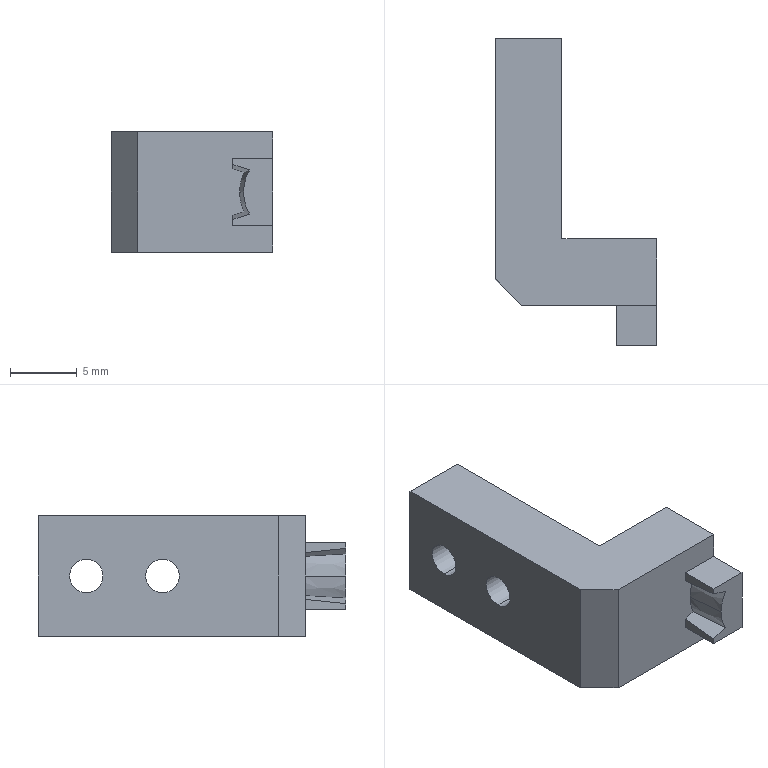Part | STEP file | PN_0015 | 1 solid | 29 faces | box 12.1 x 23 x 9 mm | volume 1039 mm3 | plane 20 | cylinder 7 | cone 2 | commonest cylinder face diameters 2.5 x4 2 x3